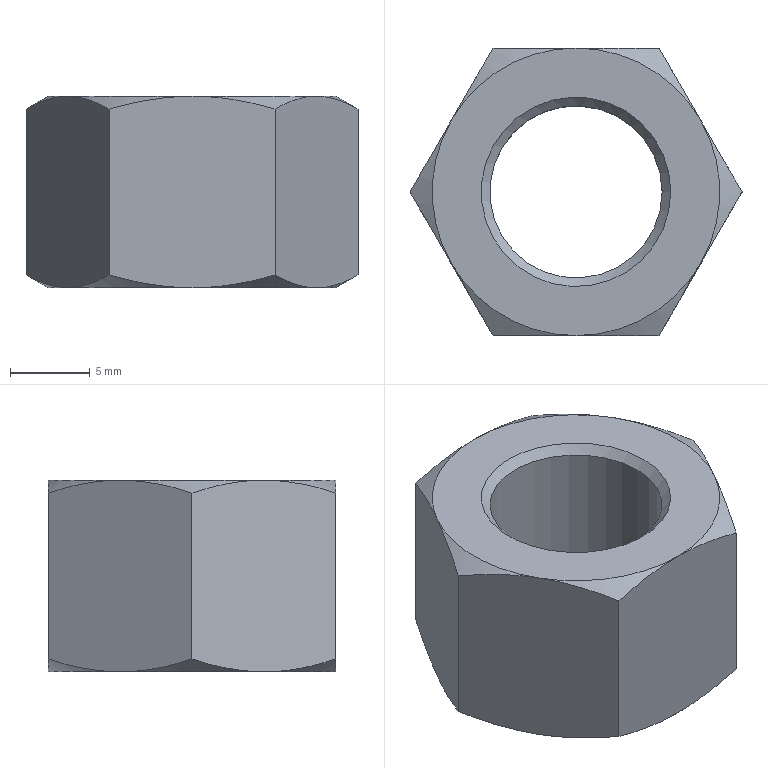Part | NX | features META 3, SKETCH 3, DATUM_CSYS 2, EXTRUDE 2, SWP104 2, CHAMFER 1, LINE 1, SYMBOLIC_THREAD 1, THREADS 1 | 1 solid | 23 faces | box 20.785 x 18 x 12 mm | volume 2248 mm3 | cone 14 | plane 8 | cylinder 1 | commonest cylinder face diameters 10.782 x1
STEP:
#1=CARTESIAN_POINT('',(10.392,0.,11.196));
#2=VERTEX_POINT('',#1);
#3=CARTESIAN_POINT('',(10.392,0.,0.8038));
#4=VERTEX_POINT('',#3);
#5=CARTESIAN_POINT('',(10.392,0.,12.));
#6=DIRECTION('',(0.,0.,-1.));
#7=VECTOR('',#6,1000.);
#8=LINE('',#5,#7);
#9=EDGE_CURVE('',#2,#4,#8,.T.);
#10=ORIENTED_EDGE('',*,*,#9,.T.);
#11=CARTESIAN_POINT('',(7.794,4.5,0.));
#12=VERTEX_POINT('',#11);
#13=CARTESIAN_POINT('',(10.392,0.,0.8038));
#14=CARTESIAN_POINT('',(9.542,1.472,0.3131));
#15=CARTESIAN_POINT('',(8.679,2.967,0.));
#16=CARTESIAN_POINT('',(7.794,4.5,0.));
#17=B_SPLINE_CURVE_WITH_KNOTS('',3,(#13,#14,#15,#16),.UNSPECIFIED.,.F.,.F.,(4,4),(0.000000238,0.005258),.UNSPECIFIED.);
#18=EDGE_CURVE('',#4,#12,#17,.T.);
#19=ORIENTED_EDGE('',*,*,#18,.T.);
#20=CARTESIAN_POINT('',(5.196,9.,0.8038));
#21=VERTEX_POINT('',#20);
#22=CARTESIAN_POINT('',(7.794,4.5,0.));
#23=CARTESIAN_POINT('',(6.912,6.028,0.));
#24=CARTESIAN_POINT('',(6.044,7.531,0.3143));
#25=CARTESIAN_POINT('',(5.196,9.,0.8038));
#26=B_SPLINE_CURVE_WITH_KNOTS('',3,(#22,#23,#24,#25),.UNSPECIFIED.,.F.,.F.,(4,4),(0.005258,0.0105),.UNSPECIFIED.);
#27=EDGE_CURVE('',#12,#21,#26,.T.);
#28=ORIENTED_EDGE('',*,*,#27,.T.);
#29=CARTESIAN_POINT('',(5.196,9.,11.196));
#30=VERTEX_POINT('',#29);
#31=CARTESIAN_POINT('',(5.196,9.,12.));
#32=DIRECTION('',(0.,0.,-1.));
#33=VECTOR('',#32,1000.);
#34=LINE('',#31,#33);
#35=EDGE_CURVE('',#30,#21,#34,.T.);
#36=ORIENTED_EDGE('',*,*,#35,.F.);
#37=CARTESIAN_POINT('',(7.794,4.5,12.));
#38=VERTEX_POINT('',#37);
#39=CARTESIAN_POINT('',(5.196,9.,11.196));
#40=CARTESIAN_POINT('',(6.046,7.528,11.687));
#41=CARTESIAN_POINT('',(6.909,6.033,12.));
#42=CARTESIAN_POINT('',(7.794,4.5,12.));
#43=B_SPLINE_CURVE_WITH_KNOTS('',3,(#39,#40,#41,#42),.UNSPECIFIED.,.F.,.F.,(4,4),(0.000000238,0.005258),.UNSPECIFIED.);
#44=EDGE_CURVE('',#30,#38,#43,.T.);
#45=ORIENTED_EDGE('',*,*,#44,.T.);
#46=CARTESIAN_POINT('',(7.794,4.5,12.));
#47=CARTESIAN_POINT('',(8.676,2.972,12.));
#48=CARTESIAN_POINT('',(9.544,1.469,11.686));
#49=CARTESIAN_POINT('',(10.392,0.,11.196));
#50=B_SPLINE_CURVE_WITH_KNOTS('',3,(#46,#47,#48,#49),.UNSPECIFIED.,.F.,.F.,(4,4),(0.005258,0.0105),.UNSPECIFIED.);
#51=EDGE_CURVE('',#38,#2,#50,.T.);
#52=ORIENTED_EDGE('',*,*,#51,.T.);
#53=EDGE_LOOP('',(#10,#19,#28,#36,#45,#52));
#54=FACE_BOUND('',#53,.T.);
#55=CARTESIAN_POINT('',(5.196,9.,12.));
#56=DIRECTION('',(0.866,0.5,0.));
#57=DIRECTION('',(-0.5,0.866,0.));
#58=AXIS2_PLACEMENT_3D('',#55,#56,#57);
#59=PLANE('',#58);
#60=ADVANCED_FACE('',(#54),#59,.T.);
#61=CARTESIAN_POINT('',(5.196,-9.,11.196));
#62=VERTEX_POINT('',#61);
#63=CARTESIAN_POINT('',(5.196,-9.,0.8038));
#64=VERTEX_POINT('',#63);
#65=CARTESIAN_POINT('',(5.196,-9.,12.));
#66=DIRECTION('',(0.,0.,-1.));
#67=VECTOR('',#66,1000.);
#68=LINE('',#65,#67);
#69=EDGE_CURVE('',#62,#64,#68,.T.);
#70=ORIENTED_EDGE('',*,*,#69,.T.);
#71=CARTESIAN_POINT('',(7.794,-4.5,0.));
#72=VERTEX_POINT('',#71);
#73=CARTESIAN_POINT('',(5.196,-9.,0.8038));
#74=CARTESIAN_POINT('',(6.046,-7.528,0.3131));
#75=CARTESIAN_POINT('',(6.909,-6.033,0.));
#76=CARTESIAN_POINT('',(7.794,-4.5,0.));
#77=B_SPLINE_CURVE_WITH_KNOTS('',3,(#73,#74,#75,#76),.UNSPECIFIED.,.F.,.F.,(4,4),(0.000000238,0.005258),.UNSPECIFIED.);
#78=EDGE_CURVE('',#64,#72,#77,.T.);
#79=ORIENTED_EDGE('',*,*,#78,.T.);
#80=CARTESIAN_POINT('',(7.794,-4.5,0.));
#81=CARTESIAN_POINT('',(8.676,-2.972,0.));
#82=CARTESIAN_POINT('',(9.544,-1.469,0.3143));
#83=CARTESIAN_POINT('',(10.392,0.,0.8038));
#84=B_SPLINE_CURVE_WITH_KNOTS('',3,(#80,#81,#82,#83),.UNSPECIFIED.,.F.,.F.,(4,4),(0.005258,0.0105),.UNSPECIFIED.);
#85=EDGE_CURVE('',#72,#4,#84,.T.);
#86=ORIENTED_EDGE('',*,*,#85,.T.);
#87=ORIENTED_EDGE('',*,*,#9,.F.);
#88=CARTESIAN_POINT('',(7.794,-4.5,12.));
#89=VERTEX_POINT('',#88);
#90=CARTESIAN_POINT('',(10.392,0.,11.196));
#91=CARTESIAN_POINT('',(9.542,-1.472,11.687));
#92=CARTESIAN_POINT('',(8.679,-2.967,12.));
#93=CARTESIAN_POINT('',(7.794,-4.5,12.));
#94=B_SPLINE_CURVE_WITH_KNOTS('',3,(#90,#91,#92,#93),.UNSPECIFIED.,.F.,.F.,(4,4),(0.000000238,0.005258),.UNSPECIFIED.);
#95=EDGE_CURVE('',#2,#89,#94,.T.);
#96=ORIENTED_EDGE('',*,*,#95,.T.);
#97=CARTESIAN_POINT('',(7.794,-4.5,12.));
#98=CARTESIAN_POINT('',(6.912,-6.028,12.));
#99=CARTESIAN_POINT('',(6.044,-7.531,11.686));
#100=CARTESIAN_POINT('',(5.196,-9.,11.196));
#101=B_SPLINE_CURVE_WITH_KNOTS('',3,(#97,#98,#99,#100),.UNSPECIFIED.,.F.,.F.,(4,4),(0.005258,0.0105),.UNSPECIFIED.);
#102=EDGE_CURVE('',#89,#62,#101,.T.);
#103=ORIENTED_EDGE('',*,*,#102,.T.);
#104=EDGE_LOOP('',(#70,#79,#86,#87,#96,#103));
#105=FACE_BOUND('',#104,.T.);
#106=CARTESIAN_POINT('',(10.392,0.,12.));
#107=DIRECTION('',(0.866,-0.5,0.));
#108=DIRECTION('',(0.5,0.866,0.));
#109=AXIS2_PLACEMENT_3D('',#106,#107,#108);
#110=PLANE('',#109);
#111=ADVANCED_FACE('',(#105),#110,.T.);
#112=CARTESIAN_POINT('',(-5.196,-9.,11.196));
#113=VERTEX_POINT('',#112);
#114=CARTESIAN_POINT('',(-5.196,-9.,0.8038));
#115=VERTEX_POINT('',#114);
#116=CARTESIAN_POINT('',(-5.196,-9.,12.));
#117=DIRECTION('',(0.,0.,-1.));
#118=VECTOR('',#117,1000.);
#119=LINE('',#116,#118);
#120=EDGE_CURVE('',#113,#115,#119,.T.);
#121=ORIENTED_EDGE('',*,*,#120,.T.);
#122=CARTESIAN_POINT('',(0.,-9.,0.));
#123=VERTEX_POINT('',#122);
#124=CARTESIAN_POINT('',(-5.196,-9.,0.8038));
#125=CARTESIAN_POINT('',(-3.506,-9.,0.3159));
#126=CARTESIAN_POINT('',(-1.756,-9.,0.));
#127=CARTESIAN_POINT('',(0.,-9.,0.));
#128=B_SPLINE_CURVE_WITH_KNOTS('',3,(#124,#125,#126,#127),.UNSPECIFIED.,.F.,.F.,(4,4),(0.009271,0.01453),.UNSPECIFIED.);
#129=EDGE_CURVE('',#115,#123,#128,.T.);
#130=ORIENTED_EDGE('',*,*,#129,.T.);
#131=CARTESIAN_POINT('',(0.,-9.,0.));
#132=CARTESIAN_POINT('',(1.757,-9.,0.));
#133=CARTESIAN_POINT('',(3.516,-9.,0.3188));
#134=CARTESIAN_POINT('',(5.196,-9.,0.8038));
#135=B_SPLINE_CURVE_WITH_KNOTS('',3,(#131,#132,#133,#134),.UNSPECIFIED.,.F.,.F.,(4,4),(0.01453,0.01979),.UNSPECIFIED.);
#136=EDGE_CURVE('',#123,#64,#135,.T.);
#137=ORIENTED_EDGE('',*,*,#136,.T.);
#138=ORIENTED_EDGE('',*,*,#69,.F.);
#139=CARTESIAN_POINT('',(0.,-9.,12.));
#140=VERTEX_POINT('',#139);
#141=CARTESIAN_POINT('',(0.,-9.,12.));
#142=CARTESIAN_POINT('',(1.757,-9.,12.));
#143=CARTESIAN_POINT('',(3.516,-9.,11.681));
#144=CARTESIAN_POINT('',(5.196,-9.,11.196));
#145=B_SPLINE_CURVE_WITH_KNOTS('',3,(#141,#142,#143,#144),.UNSPECIFIED.,.F.,.F.,(4,4),(0.01453,0.01979),.UNSPECIFIED.);
#146=EDGE_CURVE('',#62,#140,#145,.F.);
#147=ORIENTED_EDGE('',*,*,#146,.T.);
#148=CARTESIAN_POINT('',(-5.196,-9.,11.196));
#149=CARTESIAN_POINT('',(-3.506,-9.,11.684));
#150=CARTESIAN_POINT('',(-1.756,-9.,12.));
#151=CARTESIAN_POINT('',(0.,-9.,12.));
#152=B_SPLINE_CURVE_WITH_KNOTS('',3,(#148,#149,#150,#151),.UNSPECIFIED.,.F.,.F.,(4,4),(0.009271,0.01453),.UNSPECIFIED.);
#153=EDGE_CURVE('',#140,#113,#152,.F.);
#154=ORIENTED_EDGE('',*,*,#153,.T.);
#155=EDGE_LOOP('',(#121,#130,#137,#138,#147,#154));
#156=FACE_BOUND('',#155,.T.);
#157=CARTESIAN_POINT('',(5.196,-9.,12.));
#158=DIRECTION('',(0.,-1.,0.));
#159=DIRECTION('',(1.,0.,0.));
#160=AXIS2_PLACEMENT_3D('',#157,#158,#159);
#161=PLANE('',#160);
#162=ADVANCED_FACE('',(#156),#161,.T.);
#163=CARTESIAN_POINT('',(-10.392,0.,11.196));
#164=VERTEX_POINT('',#163);
#165=CARTESIAN_POINT('',(-10.392,0.,0.8038));
#166=VERTEX_POINT('',#165);
#167=CARTESIAN_POINT('',(-10.392,0.,12.));
#168=DIRECTION('',(0.,0.,-1.));
#169=VECTOR('',#168,1000.);
#170=LINE('',#167,#169);
#171=EDGE_CURVE('',#164,#166,#170,.T.);
#172=ORIENTED_EDGE('',*,*,#171,.T.);
#173=CARTESIAN_POINT('',(-7.794,-4.5,0.));
#174=VERTEX_POINT('',#173);
#175=CARTESIAN_POINT('',(-10.392,0.,0.8038));
#176=CARTESIAN_POINT('',(-9.542,-1.472,0.3131));
#177=CARTESIAN_POINT('',(-8.679,-2.967,0.));
#178=CARTESIAN_POINT('',(-7.794,-4.5,0.));
#179=B_SPLINE_CURVE_WITH_KNOTS('',3,(#175,#176,#177,#178),.UNSPECIFIED.,.F.,.F.,(4,4),(0.000000238,0.005258),.UNSPECIFIED.);
#180=EDGE_CURVE('',#166,#174,#179,.T.);
#181=ORIENTED_EDGE('',*,*,#180,.T.);
#182=CARTESIAN_POINT('',(-7.794,-4.5,0.));
#183=CARTESIAN_POINT('',(-6.912,-6.028,0.));
#184=CARTESIAN_POINT('',(-6.044,-7.531,0.3143));
#185=CARTESIAN_POINT('',(-5.196,-9.,0.8038));
#186=B_SPLINE_CURVE_WITH_KNOTS('',3,(#182,#183,#184,#185),.UNSPECIFIED.,.F.,.F.,(4,4),(0.005258,0.0105),.UNSPECIFIED.);
#187=EDGE_CURVE('',#174,#115,#186,.T.);
#188=ORIENTED_EDGE('',*,*,#187,.T.);
#189=ORIENTED_EDGE('',*,*,#120,.F.);
#190=CARTESIAN_POINT('',(-7.794,-4.5,12.));
#191=VERTEX_POINT('',#190);
#192=CARTESIAN_POINT('',(-5.196,-9.,11.196));
#193=CARTESIAN_POINT('',(-6.046,-7.528,11.687));
#194=CARTESIAN_POINT('',(-6.909,-6.033,12.));
#195=CARTESIAN_POINT('',(-7.794,-4.5,12.));
#196=B_SPLINE_CURVE_WITH_KNOTS('',3,(#192,#193,#194,#195),.UNSPECIFIED.,.F.,.F.,(4,4),(0.000000238,0.005258),.UNSPECIFIED.);
#197=EDGE_CURVE('',#113,#191,#196,.T.);
#198=ORIENTED_EDGE('',*,*,#197,.T.);
#199=CARTESIAN_POINT('',(-7.794,-4.5,12.));
#200=CARTESIAN_POINT('',(-8.676,-2.972,12.));
#201=CARTESIAN_POINT('',(-9.544,-1.469,11.686));
#202=CARTESIAN_POINT('',(-10.392,0.,11.196));
#203=B_SPLINE_CURVE_WITH_KNOTS('',3,(#199,#200,#201,#202),.UNSPECIFIED.,.F.,.F.,(4,4),(0.005258,0.0105),.UNSPECIFIED.);
#204=EDGE_CURVE('',#191,#164,#203,.T.);
#205=ORIENTED_EDGE('',*,*,#204,.T.);
#206=EDGE_LOOP('',(#172,#181,#188,#189,#198,#205));
#207=FACE_BOUND('',#206,.T.);
#208=CARTESIAN_POINT('',(-5.196,-9.,12.));
#209=DIRECTION('',(-0.866,-0.5,0.));
#210=DIRECTION('',(0.5,-0.866,0.));
#211=AXIS2_PLACEMENT_3D('',#208,#209,#210);
#212=PLANE('',#211);
#213=ADVANCED_FACE('',(#207),#212,.T.);
#214=CARTESIAN_POINT('',(-5.196,9.,11.196));
#215=VERTEX_POINT('',#214);
#216=CARTESIAN_POINT('',(-5.196,9.,0.8038));
#217=VERTEX_POINT('',#216);
#218=CARTESIAN_POINT('',(-5.196,9.,12.));
#219=DIRECTION('',(0.,0.,-1.));
#220=VECTOR('',#219,1000.);
#221=LINE('',#218,#220);
#222=EDGE_CURVE('',#215,#217,#221,.T.);
#223=ORIENTED_EDGE('',*,*,#222,.T.);
#224=CARTESIAN_POINT('',(-7.794,4.5,0.));
#225=VERTEX_POINT('',#224);
#226=CARTESIAN_POINT('',(-5.196,9.,0.8038));
#227=CARTESIAN_POINT('',(-6.046,7.528,0.3131));
#228=CARTESIAN_POINT('',(-6.909,6.033,0.));
#229=CARTESIAN_POINT('',(-7.794,4.5,0.));
#230=B_SPLINE_CURVE_WITH_KNOTS('',3,(#226,#227,#228,#229),.UNSPECIFIED.,.F.,.F.,(4,4),(0.000000238,0.005258),.UNSPECIFIED.);
#231=EDGE_CURVE('',#217,#225,#230,.T.);
#232=ORIENTED_EDGE('',*,*,#231,.T.);
#233=CARTESIAN_POINT('',(-7.794,4.5,0.));
#234=CARTESIAN_POINT('',(-8.676,2.972,0.));
#235=CARTESIAN_POINT('',(-9.544,1.469,0.3143));
#236=CARTESIAN_POINT('',(-10.392,0.,0.8038));
#237=B_SPLINE_CURVE_WITH_KNOTS('',3,(#233,#234,#235,#236),.UNSPECIFIED.,.F.,.F.,(4,4),(0.005258,0.0105),.UNSPECIFIED.);
#238=EDGE_CURVE('',#225,#166,#237,.T.);
#239=ORIENTED_EDGE('',*,*,#238,.T.);
#240=ORIENTED_EDGE('',*,*,#171,.F.);
#241=CARTESIAN_POINT('',(-7.794,4.5,12.));
#242=VERTEX_POINT('',#241);
#243=CARTESIAN_POINT('',(-10.392,0.,11.196));
#244=CARTESIAN_POINT('',(-9.542,1.472,11.687));
#245=CARTESIAN_POINT('',(-8.679,2.967,12.));
#246=CARTESIAN_POINT('',(-7.794,4.5,12.));
#247=B_SPLINE_CURVE_WITH_KNOTS('',3,(#243,#244,#245,#246),.UNSPECIFIED.,.F.,.F.,(4,4),(0.000000238,0.005258),.UNSPECIFIED.);
#248=EDGE_CURVE('',#164,#242,#247,.T.);
#249=ORIENTED_EDGE('',*,*,#248,.T.);
#250=CARTESIAN_POINT('',(-7.794,4.5,12.));
#251=CARTESIAN_POINT('',(-6.912,6.028,12.));
#252=CARTESIAN_POINT('',(-6.044,7.531,11.686));
#253=CARTESIAN_POINT('',(-5.196,9.,11.196));
#254=B_SPLINE_CURVE_WITH_KNOTS('',3,(#250,#251,#252,#253),.UNSPECIFIED.,.F.,.F.,(4,4),(0.005258,0.0105),.UNSPECIFIED.);
#255=EDGE_CURVE('',#242,#215,#254,.T.);
#256=ORIENTED_EDGE('',*,*,#255,.T.);
#257=EDGE_LOOP('',(#223,#232,#239,#240,#249,#256));
#258=FACE_BOUND('',#257,.T.);
#259=CARTESIAN_POINT('',(-10.392,0.,12.));
#260=DIRECTION('',(-0.866,0.5,0.));
#261=DIRECTION('',(-0.5,-0.866,0.));
#262=AXIS2_PLACEMENT_3D('',#259,#260,#261);
#263=PLANE('',#262);
#264=ADVANCED_FACE('',(#258),#263,.T.);
#265=ORIENTED_EDGE('',*,*,#35,.T.);
#266=CARTESIAN_POINT('',(0.,9.,0.));
#267=VERTEX_POINT('',#266);
#268=CARTESIAN_POINT('',(0.,9.,0.));
#269=CARTESIAN_POINT('',(1.757,9.,0.));
#270=CARTESIAN_POINT('',(3.516,9.,0.3188));
#271=CARTESIAN_POINT('',(5.196,9.,0.8038));
#272=B_SPLINE_CURVE_WITH_KNOTS('',3,(#268,#269,#270,#271),.UNSPECIFIED.,.F.,.F.,(4,4),(0.01453,0.01979),.UNSPECIFIED.);
#273=EDGE_CURVE('',#21,#267,#272,.F.);
#274=ORIENTED_EDGE('',*,*,#273,.T.);
#275=CARTESIAN_POINT('',(-5.196,9.,0.8038));
#276=CARTESIAN_POINT('',(-3.506,9.,0.3159));
#277=CARTESIAN_POINT('',(-1.756,9.,0.));
#278=CARTESIAN_POINT('',(0.,9.,0.));
#279=B_SPLINE_CURVE_WITH_KNOTS('',3,(#275,#276,#277,#278),.UNSPECIFIED.,.F.,.F.,(4,4),(0.009271,0.01453),.UNSPECIFIED.);
#280=EDGE_CURVE('',#267,#217,#279,.F.);
#281=ORIENTED_EDGE('',*,*,#280,.T.);
#282=ORIENTED_EDGE('',*,*,#222,.F.);
#283=CARTESIAN_POINT('',(0.,9.,12.));
#284=VERTEX_POINT('',#283);
#285=CARTESIAN_POINT('',(-5.196,9.,11.196));
#286=CARTESIAN_POINT('',(-3.506,9.,11.684));
#287=CARTESIAN_POINT('',(-1.756,9.,12.));
#288=CARTESIAN_POINT('',(0.,9.,12.));
#289=B_SPLINE_CURVE_WITH_KNOTS('',3,(#285,#286,#287,#288),.UNSPECIFIED.,.F.,.F.,(4,4),(0.009271,0.01453),.UNSPECIFIED.);
#290=EDGE_CURVE('',#215,#284,#289,.T.);
#291=ORIENTED_EDGE('',*,*,#290,.T.);
#292=CARTESIAN_POINT('',(0.,9.,12.));
#293=CARTESIAN_POINT('',(1.757,9.,12.));
#294=CARTESIAN_POINT('',(3.516,9.,11.681));
#295=CARTESIAN_POINT('',(5.196,9.,11.196));
#296=B_SPLINE_CURVE_WITH_KNOTS('',3,(#292,#293,#294,#295),.UNSPECIFIED.,.F.,.F.,(4,4),(0.01453,0.01979),.UNSPECIFIED.);
#297=EDGE_CURVE('',#284,#30,#296,.T.);
#298=ORIENTED_EDGE('',*,*,#297,.T.);
#299=EDGE_LOOP('',(#265,#274,#281,#282,#291,#298));
#300=FACE_BOUND('',#299,.T.);
#301=CARTESIAN_POINT('',(-5.196,9.,12.));
#302=DIRECTION('',(0.,1.,0.));
#303=DIRECTION('',(0.,0.,1.));
#304=AXIS2_PLACEMENT_3D('',#301,#302,#303);
#305=PLANE('',#304);
#306=ADVANCED_FACE('',(#300),#305,.T.);
#307=ORIENTED_EDGE('',*,*,#297,.F.);
#308=CARTESIAN_POINT('',(0.,0.,12.));
#309=DIRECTION('',(0.,0.,-1.));
#310=DIRECTION('',(-1.,0.,0.));
#311=AXIS2_PLACEMENT_3D('',#308,#309,#310);
#312=CIRCLE('',#311,9.);
#313=EDGE_CURVE('',#284,#38,#312,.T.);
#314=ORIENTED_EDGE('',*,*,#313,.T.);
#315=ORIENTED_EDGE('',*,*,#44,.F.);
#316=EDGE_LOOP('',(#307,#314,#315));
#317=FACE_BOUND('',#316,.T.);
#318=CARTESIAN_POINT('',(0.,0.,11.196));
#319=DIRECTION('',(0.,0.,-1.));
#320=DIRECTION('',(-1.,0.,0.));
#321=AXIS2_PLACEMENT_3D('',#318,#319,#320);
#322=CONICAL_SURFACE('',#321,10.392,1.047);
#323=ADVANCED_FACE('',(#317),#322,.T.);
#324=CARTESIAN_POINT('',(0.,0.,12.));
#325=DIRECTION('',(0.,0.,-1.));
#326=DIRECTION('',(-1.,0.,0.));
#327=AXIS2_PLACEMENT_3D('',#324,#325,#326);
#328=CIRCLE('',#327,9.);
#329=EDGE_CURVE('',#242,#284,#328,.T.);
#330=ORIENTED_EDGE('',*,*,#329,.T.);
#331=ORIENTED_EDGE('',*,*,#290,.F.);
#332=ORIENTED_EDGE('',*,*,#255,.F.);
#333=EDGE_LOOP('',(#330,#331,#332));
#334=FACE_BOUND('',#333,.T.);
#335=CARTESIAN_POINT('',(0.,0.,11.196));
#336=DIRECTION('',(0.,0.,-1.));
#337=DIRECTION('',(-1.,0.,0.));
#338=AXIS2_PLACEMENT_3D('',#335,#336,#337);
#339=CONICAL_SURFACE('',#338,10.392,1.047);
#340=ADVANCED_FACE('',(#334),#339,.T.);
#341=CARTESIAN_POINT('',(0.,0.,12.));
#342=DIRECTION('',(0.,0.,-1.));
#343=DIRECTION('',(-1.,0.,0.));
#344=AXIS2_PLACEMENT_3D('',#341,#342,#343);
#345=CIRCLE('',#344,9.);
#346=EDGE_CURVE('',#191,#242,#345,.T.);
#347=ORIENTED_EDGE('',*,*,#346,.T.);
#348=ORIENTED_EDGE('',*,*,#248,.F.);
#349=ORIENTED_EDGE('',*,*,#204,.F.);
#350=EDGE_LOOP('',(#347,#348,#349));
#351=FACE_BOUND('',#350,.T.);
#352=CARTESIAN_POINT('',(0.,0.,11.196));
#353=DIRECTION('',(0.,0.,-1.));
#354=DIRECTION('',(-1.,0.,0.));
#355=AXIS2_PLACEMENT_3D('',#352,#353,#354);
#356=CONICAL_SURFACE('',#355,10.392,1.047);
#357=ADVANCED_FACE('',(#351),#356,.T.);
#358=CARTESIAN_POINT('',(0.,0.,12.));
#359=DIRECTION('',(0.,0.,-1.));
#360=DIRECTION('',(-1.,0.,0.));
#361=AXIS2_PLACEMENT_3D('',#358,#359,#360);
#362=CIRCLE('',#361,9.);
#363=EDGE_CURVE('',#140,#191,#362,.T.);
#364=ORIENTED_EDGE('',*,*,#363,.T.);
#365=ORIENTED_EDGE('',*,*,#197,.F.);
#366=ORIENTED_EDGE('',*,*,#153,.F.);
#367=EDGE_LOOP('',(#364,#365,#366));
#368=FACE_BOUND('',#367,.T.);
#369=CARTESIAN_POINT('',(0.,0.,11.196));
#370=DIRECTION('',(0.,0.,-1.));
#371=DIRECTION('',(-1.,0.,0.));
#372=AXIS2_PLACEMENT_3D('',#369,#370,#371);
#373=CONICAL_SURFACE('',#372,10.392,1.047);
#374=ADVANCED_FACE('',(#368),#373,.T.);
#375=CARTESIAN_POINT('',(0.,0.,12.));
#376=DIRECTION('',(0.,0.,-1.));
#377=DIRECTION('',(-1.,0.,0.));
#378=AXIS2_PLACEMENT_3D('',#375,#376,#377);
#379=CIRCLE('',#378,9.);
#380=EDGE_CURVE('',#89,#140,#379,.T.);
#381=ORIENTED_EDGE('',*,*,#380,.T.);
#382=ORIENTED_EDGE('',*,*,#146,.F.);
#383=ORIENTED_EDGE('',*,*,#102,.F.);
#384=EDGE_LOOP('',(#381,#382,#383));
#385=FACE_BOUND('',#384,.T.);
#386=CARTESIAN_POINT('',(0.,0.,11.196));
#387=DIRECTION('',(0.,0.,-1.));
#388=DIRECTION('',(-1.,0.,0.));
#389=AXIS2_PLACEMENT_3D('',#386,#387,#388);
#390=CONICAL_SURFACE('',#389,10.392,1.047);
#391=ADVANCED_FACE('',(#385),#390,.T.);
#392=CARTESIAN_POINT('',(0.,0.,12.));
#393=DIRECTION('',(0.,0.,-1.));
#394=DIRECTION('',(-1.,0.,0.));
#395=AXIS2_PLACEMENT_3D('',#392,#393,#394);
#396=CIRCLE('',#395,9.);
#397=EDGE_CURVE('',#38,#89,#396,.T.);
#398=ORIENTED_EDGE('',*,*,#397,.T.);
#399=ORIENTED_EDGE('',*,*,#95,.F.);
#400=ORIENTED_EDGE('',*,*,#51,.F.);
#401=EDGE_LOOP('',(#398,#399,#400));
#402=FACE_BOUND('',#401,.T.);
#403=CARTESIAN_POINT('',(0.,0.,11.196));
#404=DIRECTION('',(0.,0.,-1.));
#405=DIRECTION('',(-1.,0.,0.));
#406=AXIS2_PLACEMENT_3D('',#403,#404,#405);
#407=CONICAL_SURFACE('',#406,10.392,1.047);
#408=ADVANCED_FACE('',(#402),#407,.T.);
#409=CARTESIAN_POINT('',(5.93,0.,12.));
#410=VERTEX_POINT('',#409);
#411=CARTESIAN_POINT('',(0.,0.,12.));
#412=DIRECTION('',(0.,0.,1.));
#413=DIRECTION('',(1.,0.,0.));
#414=AXIS2_PLACEMENT_3D('',#411,#412,#413);
#415=CIRCLE('',#414,5.93);
#416=EDGE_CURVE('',#410,#410,#415,.F.);
#417=ORIENTED_EDGE('',*,*,#416,.T.);
#418=EDGE_LOOP('',(#417));
#419=FACE_BOUND('',#418,.T.);
#420=ORIENTED_EDGE('',*,*,#329,.F.);
#421=ORIENTED_EDGE('',*,*,#346,.F.);
#422=ORIENTED_EDGE('',*,*,#363,.F.);
#423=ORIENTED_EDGE('',*,*,#380,.F.);
#424=ORIENTED_EDGE('',*,*,#397,.F.);
#425=ORIENTED_EDGE('',*,*,#313,.F.);
#426=EDGE_LOOP('',(#420,#421,#422,#423,#424,#425));
#427=FACE_BOUND('',#426,.T.);
#428=CARTESIAN_POINT('',(0.,18.,12.));
#429=DIRECTION('',(0.,0.,1.));
#430=DIRECTION('',(1.,0.,0.));
#431=AXIS2_PLACEMENT_3D('',#428,#429,#430);
#432=PLANE('',#431);
#433=ADVANCED_FACE('',(#419,#427),#432,.T.);
#434=ORIENTED_EDGE('',*,*,#280,.F.);
#435=CARTESIAN_POINT('',(0.,0.,0.));
#436=DIRECTION('',(0.,0.,-1.));
#437=DIRECTION('',(-1.,0.,0.));
#438=AXIS2_PLACEMENT_3D('',#435,#436,#437);
#439=CIRCLE('',#438,9.);
#440=EDGE_CURVE('',#225,#267,#439,.T.);
#441=ORIENTED_EDGE('',*,*,#440,.F.);
#442=ORIENTED_EDGE('',*,*,#231,.F.);
#443=EDGE_LOOP('',(#434,#441,#442));
#444=FACE_BOUND('',#443,.T.);
#445=CARTESIAN_POINT('',(0.,0.,0.));
#446=DIRECTION('',(0.,0.,1.));
#447=DIRECTION('',(1.,0.,0.));
#448=AXIS2_PLACEMENT_3D('',#445,#446,#447);
#449=CONICAL_SURFACE('',#448,9.,1.047);
#450=ADVANCED_FACE('',(#444),#449,.T.);
#451=CARTESIAN_POINT('',(0.,0.,0.));
#452=DIRECTION('',(0.,0.,-1.));
#453=DIRECTION('',(-1.,0.,0.));
#454=AXIS2_PLACEMENT_3D('',#451,#452,#453);
#455=CIRCLE('',#454,9.);
#456=EDGE_CURVE('',#267,#12,#455,.T.);
#457=ORIENTED_EDGE('',*,*,#456,.F.);
#458=ORIENTED_EDGE('',*,*,#273,.F.);
#459=ORIENTED_EDGE('',*,*,#27,.F.);
#460=EDGE_LOOP('',(#457,#458,#459));
#461=FACE_BOUND('',#460,.T.);
#462=CARTESIAN_POINT('',(0.,0.,0.));
#463=DIRECTION('',(0.,0.,1.));
#464=DIRECTION('',(1.,0.,0.));
#465=AXIS2_PLACEMENT_3D('',#462,#463,#464);
#466=CONICAL_SURFACE('',#465,9.,1.047);
#467=ADVANCED_FACE('',(#461),#466,.T.);
#468=ORIENTED_EDGE('',*,*,#238,.F.);
#469=CARTESIAN_POINT('',(0.,0.,0.));
#470=DIRECTION('',(0.,0.,-1.));
#471=DIRECTION('',(-1.,0.,0.));
#472=AXIS2_PLACEMENT_3D('',#469,#470,#471);
#473=CIRCLE('',#472,9.);
#474=EDGE_CURVE('',#174,#225,#473,.T.);
#475=ORIENTED_EDGE('',*,*,#474,.F.);
#476=ORIENTED_EDGE('',*,*,#180,.F.);
#477=EDGE_LOOP('',(#468,#475,#476));
#478=FACE_BOUND('',#477,.T.);
#479=CARTESIAN_POINT('',(0.,0.,0.));
#480=DIRECTION('',(0.,0.,1.));
#481=DIRECTION('',(1.,0.,0.));
#482=AXIS2_PLACEMENT_3D('',#479,#480,#481);
#483=CONICAL_SURFACE('',#482,9.,1.047);
#484=ADVANCED_FACE('',(#478),#483,.T.);
#485=ORIENTED_EDGE('',*,*,#187,.F.);
#486=CARTESIAN_POINT('',(0.,0.,0.));
#487=DIRECTION('',(0.,0.,-1.));
#488=DIRECTION('',(-1.,0.,0.));
#489=AXIS2_PLACEMENT_3D('',#486,#487,#488);
#490=CIRCLE('',#489,9.);
#491=EDGE_CURVE('',#123,#174,#490,.T.);
#492=ORIENTED_EDGE('',*,*,#491,.F.);
#493=ORIENTED_EDGE('',*,*,#129,.F.);
#494=EDGE_LOOP('',(#485,#492,#493));
#495=FACE_BOUND('',#494,.T.);
#496=CARTESIAN_POINT('',(0.,0.,0.));
#497=DIRECTION('',(0.,0.,1.));
#498=DIRECTION('',(1.,0.,0.));
#499=AXIS2_PLACEMENT_3D('',#496,#497,#498);
#500=CONICAL_SURFACE('',#499,9.,1.047);
#501=ADVANCED_FACE('',(#495),#500,.T.);
#502=CARTESIAN_POINT('',(0.,0.,0.));
#503=DIRECTION('',(0.,0.,-1.));
#504=DIRECTION('',(-1.,0.,0.));
#505=AXIS2_PLACEMENT_3D('',#502,#503,#504);
#506=CIRCLE('',#505,9.);
#507=EDGE_CURVE('',#72,#123,#506,.T.);
#508=ORIENTED_EDGE('',*,*,#507,.F.);
#509=ORIENTED_EDGE('',*,*,#78,.F.);
#510=ORIENTED_EDGE('',*,*,#136,.F.);
#511=EDGE_LOOP('',(#508,#509,#510));
#512=FACE_BOUND('',#511,.T.);
#513=CARTESIAN_POINT('',(0.,0.,0.));
#514=DIRECTION('',(0.,0.,1.));
#515=DIRECTION('',(1.,0.,0.));
#516=AXIS2_PLACEMENT_3D('',#513,#514,#515);
#517=CONICAL_SURFACE('',#516,9.,1.047);
#518=ADVANCED_FACE('',(#512),#517,.T.);
#519=CARTESIAN_POINT('',(0.,0.,0.));
#520=DIRECTION('',(0.,0.,-1.));
#521=DIRECTION('',(-1.,0.,0.));
#522=AXIS2_PLACEMENT_3D('',#519,#520,#521);
#523=CIRCLE('',#522,9.);
#524=EDGE_CURVE('',#12,#72,#523,.T.);
#525=ORIENTED_EDGE('',*,*,#524,.F.);
#526=ORIENTED_EDGE('',*,*,#18,.F.);
#527=ORIENTED_EDGE('',*,*,#85,.F.);
#528=EDGE_LOOP('',(#525,#526,#527));
#529=FACE_BOUND('',#528,.T.);
#530=CARTESIAN_POINT('',(0.,0.,0.));
#531=DIRECTION('',(0.,0.,1.));
#532=DIRECTION('',(1.,0.,0.));
#533=AXIS2_PLACEMENT_3D('',#530,#531,#532);
#534=CONICAL_SURFACE('',#533,9.,1.047);
#535=ADVANCED_FACE('',(#529),#534,.T.);
#536=CARTESIAN_POINT('',(5.93,0.,0.));
#537=VERTEX_POINT('',#536);
#538=CARTESIAN_POINT('',(0.,0.,0.));
#539=DIRECTION('',(0.,0.,1.));
#540=DIRECTION('',(1.,0.,0.));
#541=AXIS2_PLACEMENT_3D('',#538,#539,#540);
#542=CIRCLE('',#541,5.93);
#543=EDGE_CURVE('',#537,#537,#542,.T.);
#544=ORIENTED_EDGE('',*,*,#543,.T.);
#545=EDGE_LOOP('',(#544));
#546=FACE_BOUND('',#545,.T.);
#547=ORIENTED_EDGE('',*,*,#474,.T.);
#548=ORIENTED_EDGE('',*,*,#440,.T.);
#549=ORIENTED_EDGE('',*,*,#456,.T.);
#550=ORIENTED_EDGE('',*,*,#524,.T.);
#551=ORIENTED_EDGE('',*,*,#507,.T.);
#552=ORIENTED_EDGE('',*,*,#491,.T.);
#553=EDGE_LOOP('',(#547,#548,#549,#550,#551,#552));
#554=FACE_BOUND('',#553,.T.);
#555=CARTESIAN_POINT('',(0.,18.,0.));
#556=DIRECTION('',(0.,0.,1.));
#557=DIRECTION('',(1.,0.,0.));
#558=AXIS2_PLACEMENT_3D('',#555,#556,#557);
#559=PLANE('',#558);
#560=ADVANCED_FACE('',(#546,#554),#559,.F.);
#561=CARTESIAN_POINT('',(5.391,0.,0.5391));
#562=VERTEX_POINT('',#561);
#563=CARTESIAN_POINT('',(0.,0.,0.5391));
#564=DIRECTION('',(0.,0.,1.));
#565=DIRECTION('',(1.,0.,0.));
#566=AXIS2_PLACEMENT_3D('',#563,#564,#565);
#567=CIRCLE('',#566,5.391);
#568=EDGE_CURVE('',#562,#562,#567,.F.);
#569=ORIENTED_EDGE('',*,*,#568,.T.);
#570=EDGE_LOOP('',(#569));
#571=FACE_BOUND('',#570,.T.);
#572=CARTESIAN_POINT('',(5.391,0.,11.461));
#573=VERTEX_POINT('',#572);
#574=CARTESIAN_POINT('',(0.,0.,11.461));
#575=DIRECTION('',(0.,0.,1.));
#576=DIRECTION('',(1.,0.,0.));
#577=AXIS2_PLACEMENT_3D('',#574,#575,#576);
#578=CIRCLE('',#577,5.391);
#579=EDGE_CURVE('',#573,#573,#578,.T.);
#580=ORIENTED_EDGE('',*,*,#579,.T.);
#581=EDGE_LOOP('',(#580));
#582=FACE_BOUND('',#581,.T.);
#583=CARTESIAN_POINT('',(0.,0.,12.));
#584=DIRECTION('',(0.,0.,-1.));
#585=DIRECTION('',(-1.,0.,0.));
#586=AXIS2_PLACEMENT_3D('',#583,#584,#585);
#587=CYLINDRICAL_SURFACE('',#586,5.391);
#588=ADVANCED_FACE('',(#571,#582),#587,.F.);
#589=ORIENTED_EDGE('',*,*,#543,.F.);
#590=EDGE_LOOP('',(#589));
#591=FACE_BOUND('',#590,.T.);
#592=ORIENTED_EDGE('',*,*,#568,.F.);
#593=EDGE_LOOP('',(#592));
#594=FACE_BOUND('',#593,.T.);
#595=CARTESIAN_POINT('',(0.,0.,0.5391));
#596=DIRECTION('',(0.,0.,-1.));
#597=DIRECTION('',(-1.,0.,0.));
#598=AXIS2_PLACEMENT_3D('',#595,#596,#597);
#599=CONICAL_SURFACE('',#598,5.391,0.7854);
#600=ADVANCED_FACE('',(#591,#594),#599,.F.);
#601=ORIENTED_EDGE('',*,*,#579,.F.);
#602=EDGE_LOOP('',(#601));
#603=FACE_BOUND('',#602,.T.);
#604=ORIENTED_EDGE('',*,*,#416,.F.);
#605=EDGE_LOOP('',(#604));
#606=FACE_BOUND('',#605,.T.);
#607=CARTESIAN_POINT('',(0.,0.,12.));
#608=DIRECTION('',(0.,0.,1.));
#609=DIRECTION('',(1.,0.,0.));
#610=AXIS2_PLACEMENT_3D('',#607,#608,#609);
#611=CONICAL_SURFACE('',#610,5.93,0.7854);
#612=ADVANCED_FACE('',(#603,#606),#611,.F.);
#613=CLOSED_SHELL('',(#60,#111,#162,#213,#264,#306,#323,#340,#357,#374,#391,#408,#433,#450,#467,#484,#501,#518,#535,#560,#588,#600,#612));
#614=MANIFOLD_SOLID_BREP('',#613);
#615=(LENGTH_UNIT()NAMED_UNIT(*)SI_UNIT(.MILLI.,.METRE.));
#616=UNCERTAINTY_MEASURE_WITH_UNIT(LENGTH_MEASURE(0.0508),#615,'','');
#617=(NAMED_UNIT(*)PLANE_ANGLE_UNIT()SI_UNIT($,.RADIAN.));
#618=(NAMED_UNIT(*)SI_UNIT($,.STERADIAN.)SOLID_ANGLE_UNIT());
#619=(GEOMETRIC_REPRESENTATION_CONTEXT(3)GLOBAL_UNCERTAINTY_ASSIGNED_CONTEXT((#616))GLOBAL_UNIT_ASSIGNED_CONTEXT((#615,#617,#618))REPRESENTATION_CONTEXT('',''));
#620=ADVANCED_BREP_SHAPE_REPRESENTATION('',(#614),#619);